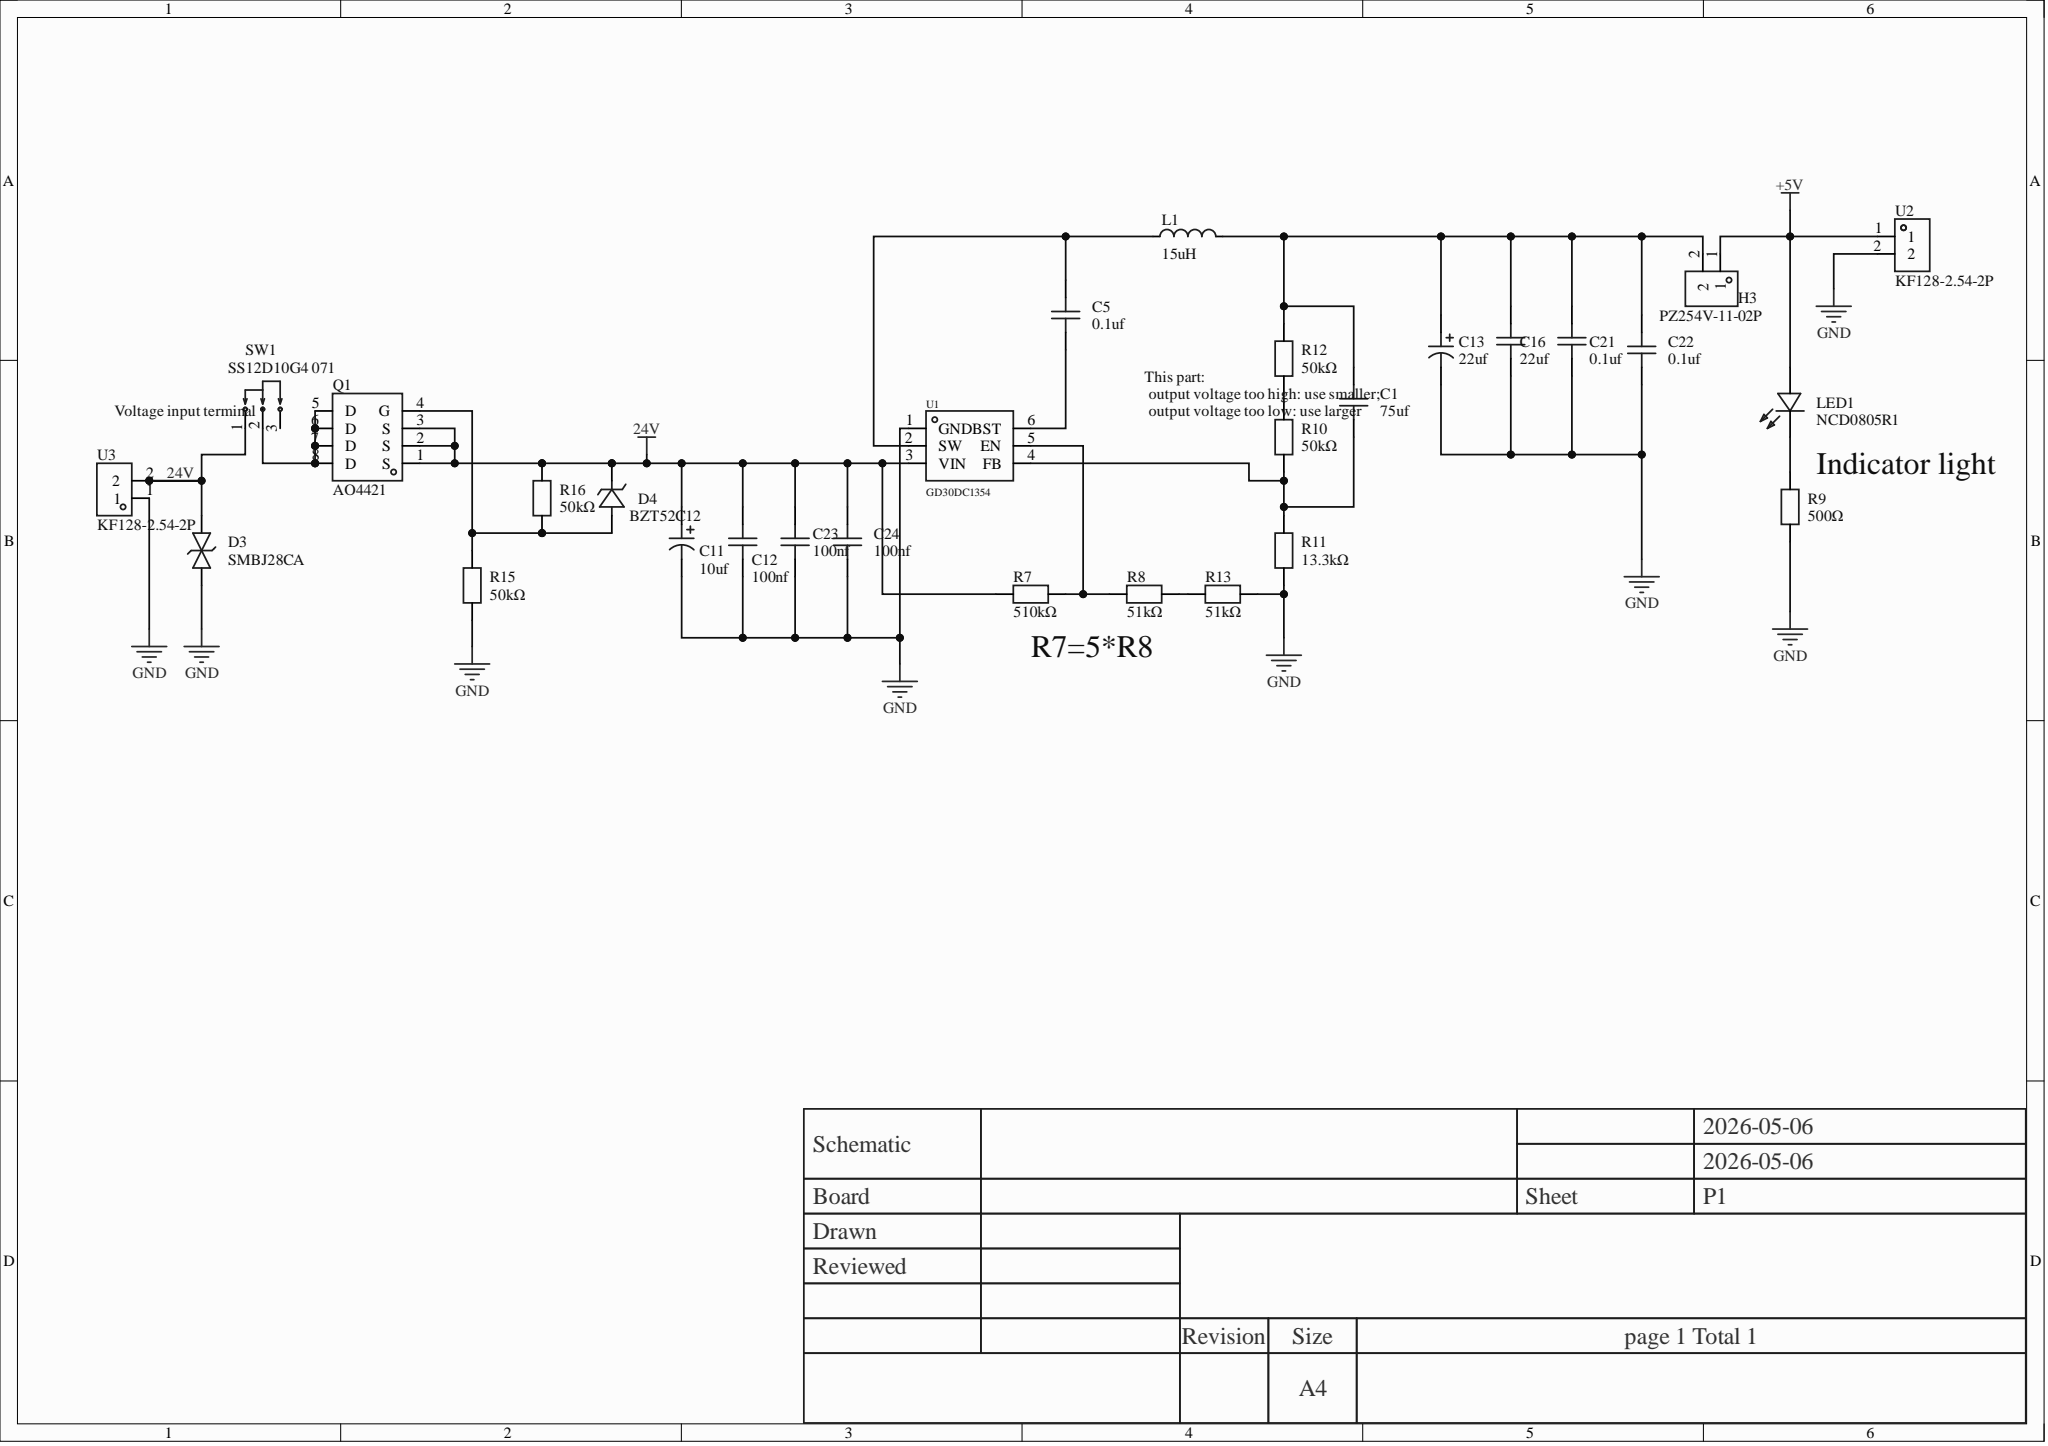Circuit board | Altium Designer | 29 parts | 13 nets
Bill of materials:
Comment,Description,Designator,Footprint,LibRef,Quantity
"75uf","Capacitance:100nF;Tolerance:±10%;Rated voltage:50V;Temperature coefficient:X7R;","C1","C0603","CGA0603X7R104K500JT","1"
"0.1uf","Capacitance:22uF;Tolerance:±20%;Rated voltage:6.3V;Temperature coefficient:X5R;","C5, C21, C22","C0603","CL10A226MQ8NRNC","3"
"10uf","Capacitance:220uF;Tolerance:±20%;Rated voltage:16V;Ripple current:110mA@120Hz;Equivalent series resistance (ESR):-;","C11","CAP-SMD_BD6.3-L6.6-W6.6-FD","RVT220UF16V67RV0015","1"
"100nf","Capacitance:100nF;Tolerance:±20%;Rated voltage:50V;Temperature coefficient:Y5V;","C12","CAP-TH_L5.0-W2.5-P5.00-D1.0","CC1H104MC1FD3F6C10MF","1"
"22uf","Capacitance:220uF;Tolerance:±20%;Rated voltage:16V;Ripple current:110mA@120Hz;Equivalent series resistance (ESR):-;","C13","CAP-SMD_BD6.3-L6.6-W6.6-FD","RVT220UF16V67RV0015","1"
"22uf","Capacitance:100nF;Tolerance:±20%;Rated voltage:50V;Temperature coefficient:Y5V;","C16","CAP-TH_L5.0-W2.5-P5.00-D1.0","CC1H104MC1FD3F6C10MF","1"
"100nf","Capacitance:22uF;Tolerance:±20%;Rated voltage:6.3V;Temperature coefficient:X5R;","C23, C24","C0603","CL10A226MQ8NRNC","2"
"SMBJ28CA","","D3","SMB_L4.6-W3.6-LS5.4-BI","SMBJ28CA_C19077583","1"
"BZT52C12","Diode configuration:Discrete;Zener voltage (nominal):12V;Zener voltage (range):11.4V~12.6V;Power dissipation (Pd):350mW;","D4","SOD-123_L2.7-W1.6-LS3.7-RD","BZT52C12_C19077410","1"
"PZ254V-11-02P","","H3","HDR-TH_2P-P2.54-V-M","PZ254V-11-02P","1"
"15uH","Inductance:15uH;Tolerance:±20%;Rated current:2.5A;Saturation current (Isat):3A;Type:Molded inductor;","L1","IND-SMD_L5.7-W5.2_GSM0530","SRG0530-150-M","1"
"NCD0805R1","","LED1","LED0805-RD","NCD0805R1","1"
"AO4421","","Q1","SOIC-8_L4.9-W3.9-P1.27-LS6.0-BL","AO4421","1"
"510kΩ","Resistor type:Thick film resistor;Resistance:10kΩ;Tolerance:±1%;Power:100mW;Working voltage:75V;Temperature coefficient:±100ppm/?;","R7","R0603","FRC0603F1002TS","1"
"51kΩ","Resistor type:Thick film resistor;Resistance:10kΩ;Tolerance:±1%;Power:100mW;Working voltage:75V;Temperature coefficient:±100ppm/?;","R8, R13","R0603","FRC0603F1002TS","2"
"500Ω","Resistor type:Thick film resistor;Resistance:10kΩ;Tolerance:±1%;Power:100mW;Working voltage:75V;Temperature coefficient:±100ppm/?;","R9","R0603","FRC0603F1002TS","1"
"50kΩ","Resistor type:Thick film resistor;Resistance:10kΩ;Tolerance:±1%;Power:100mW;Working voltage:75V;Temperature coefficient:±100ppm/?;","R10, R12, R15, R16","R0603","FRC0603F1002TS","4"
"13.3kΩ","Resistor type:Thick film resistor;Resistance:10kΩ;Tolerance:±1%;Power:100mW;Working voltage:75V;Temperature coefficient:±100ppm/?;","R11","R0603","FRC0603F1002TS","1"
"SS12D10G4 071","Circuit structure:SPDT;Mounting:Through-hole;Switch color:-;Rated current:2A;Rated voltage:125V;Operating life:3 thousand cycles;","SW1","SW-TH_SHOU-HAN_SS12D10G4","SS12D10G4 071","1"
"GD30DC1354","","U1","SOT-23-6_L2.9-W1.7-P0.95-LS2.8-BL","GD30DC1354","1"
"KF128-2.54-2P","","U2, U3","CONN-TH_P2.54_KF128-2.54-2P","KF128-2.54-2P","2"
Netlist (Protel format):
[
C1
C0603
75uf



]
[
C5
C0603
0.1uf



]
[
C11
CAP-SMD_BD6.3-L6.6-W6.6-FD
10uf



]
[
C12
CAP-TH_L5.0-W2.5-P5.00-D1.0
100nf



]
[
C13
CAP-SMD_BD6.3-L6.6-W6.6-FD
22uf



]
[
C16
CAP-TH_L5.0-W2.5-P5.00-D1.0
22uf



]
[
C21
C0603
0.1uf



]
[
C22
C0603
0.1uf



]
[
C23
C0603
100nf



]
[
C24
C0603
100nf



]
[
D3
SMB_L4.6-W3.6-LS5.4-BI
SMBJ28CA



]
[
D4
SOD-123_L2.7-W1.6-LS3.7-RD
BZT52C12



]
[
H3
HDR-TH_2P-P2.54-V-M
PZ254V-11-02P



]
[
L1
IND-SMD_L5.7-W5.2_GSM0530
15uH



]
[
LED1
LED0805-RD
NCD0805R1



]
[
Q1
SOIC-8_L4.9-W3.9-P1.27-LS6.0-BL
AO4421



]
[
R7
R0603
510kΩ



]
[
R8
R0603
51kΩ



]
[
R9
R0603
500Ω



]
[
R10
R0603
50kΩ



]
[
R11
R0603
13.3kΩ



]
[
R12
R0603
50kΩ



]
[
R13
R0603
51kΩ



]
[
R15
R0603
50kΩ



]
[
R16
R0603
50kΩ



]
[
SW1
SW-TH_SHOU-HAN_SS12D10G4
SS12D10G4 071



]
[
U1
SOT-23-6_L2.9-W1.7-P0.95-LS2.8-BL
GD30DC1354



]
[
U2
CONN-TH_P2.54_KF128-2.54-2P
KF128-2.54-2P



]
[
U3
CONN-TH_P2.54_KF128-2.54-2P
KF128-2.54-2P



]
(
NetR10_2
R10-2
R12-1
)
(
NetR8_1
R8-1
R13-2
)
(
NetR7_1
R7-1
R8-2
U1-5
)
(
NetQ1_5
Q1-5
Q1-6
Q1-7
Q1-8
SW1-2
)
(
NetLED1_1
LED1-1
R9-2
)
(
NetD4_2
D4-2
Q1-4
R15-2
R16-1
)
(
NetC5_2
C5-2
U1-6
)
(
NetC5_1
C5-1
L1-1
U1-2
)
(
NetC1_2
C1-2
C13-1
C16-2
C21-1
C22-1
H3-2
L1-2
R12-2
)
(
NetC1_1
C1-1
R10-1
R11-2
U1-4
)
(
GND
C11-2
C12-1
C13-2
C16-1
C21-2
C22-2
C23-2
C24-2
D3-1
R9-1
R11-1
R13-1
R15-1
U1-1
U2-2
U3-1
)
(
+5V
H3-1
LED1-2
U2-1
)
(
24V
C11-1
C12-2
C23-1
C24-1
D3-2
D4-1
Q1-1
Q1-2
Q1-3
R7-2
R16-2
SW1-1
U1-3
U3-2
)